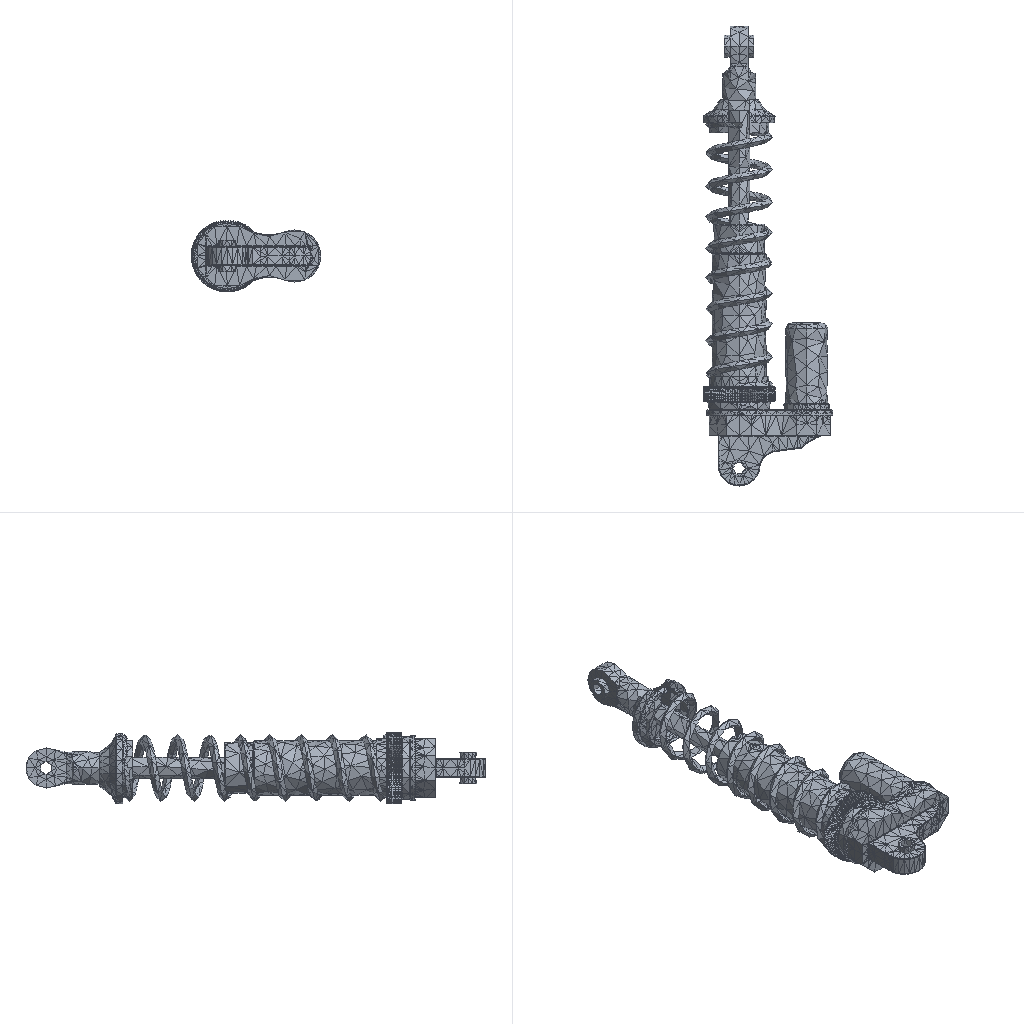Simulation study | ansys workbench
Set-up summary:
category,name,step,type,value,unit,region
solver,ansys_mapdl
solver,version,,,21.1
solver,version,,,21.1
solver,version,,,21.1
solver,version,,,21.1
solver,version,,,21.1
solver,version,,,21.1
solver,version,,,21.1
units,MPA,,stated
analysis,deck1,,transient,transient
load_step,requested,,,1
analysis,nlgeom,,,True
mesh,nodes,,,36272
mesh,elements,,,22272
element_type,ANSYS 187 (type 1),,solid,16919
element_type,ANSYS 187 (type 2),,solid,684
element_type,ANSYS 187 (type 3),,solid,554
element_type,ANSYS 187 (type 4),,solid,953
element_type,ANSYS 174 (type 5),,contact,35
element_type,ANSYS 170 (type 6),,target,35
element_type,ANSYS 174 (type 7),,contact,14
element_type,ANSYS 170 (type 8),,target,14
element_type,ANSYS 174 (type 9),,contact,1251
element_type,ANSYS 170 (type 10),,target,1251
element_type,ANSYS 174 (type 11),,contact,68
element_type,ANSYS 170 (type 12),,target,68
element_type,ANSYS 174 (type 13),,contact,148
element_type,ANSYS 170 (type 14),,target,148
element_type,ANSYS 154 (type 15),,surface,130
load,load commands in deck,,count,1
bc,support commands in deck,,count,1
named_set,_FIXEDSU,,component
analysis,deck2,,static,static
load_step,requested,,,1
analysis,nlgeom,,,False
mesh,nodes,,,36272
mesh,elements,,,22462
element_type,ANSYS 291 (type 1),,thermal_solid,16919
element_type,ANSYS 291 (type 2),,thermal_solid,684
element_type,ANSYS 291 (type 3),,thermal_solid,554
element_type,ANSYS 291 (type 4),,thermal_solid,953
element_type,ANSYS 174 (type 5),,contact,35
element_type,ANSYS 170 (type 6),,target,35
element_type,ANSYS 174 (type 7),,contact,14
element_type,ANSYS 170 (type 8),,target,14
element_type,ANSYS 174 (type 9),,contact,1251
element_type,ANSYS 170 (type 10),,target,1251
element_type,ANSYS 174 (type 11),,contact,68
element_type,ANSYS 170 (type 12),,target,68
element_type,ANSYS 174 (type 13),,contact,148
element_type,ANSYS 170 (type 14),,target,148
element_type,ANSYS 152 (type 15),,surface,320
load,load commands in deck,,count,4
bc,support commands in deck,,count,3
named_set,_CM86,,component
named_set,_CM95,,component
named_set,_ELMISC,,component
analysis,deck3,,modal,modal
load_step,requested,,,2
analysis,nlgeom,,,False
mesh,nodes,,,0
mesh,elements,,,0
load,load commands in deck,,count,0
bc,support commands in deck,,count,0
analysis,deck4,,modal,HARM; modal
load_step,requested,,,4
analysis,nlgeom,,,False
mesh,nodes,,,36272
mesh,elements,,,22272
element_type,ANSYS 187 (type 1),,solid,16919
element_type,ANSYS 187 (type 2),,solid,684
element_type,ANSYS 187 (type 3),,solid,554
element_type,ANSYS 187 (type 4),,solid,953
element_type,ANSYS 174 (type 5),,contact,35
element_type,ANSYS 170 (type 6),,target,35
element_type,ANSYS 174 (type 7),,contact,14
element_type,ANSYS 170 (type 8),,target,14
element_type,ANSYS 174 (type 9),,contact,1251
element_type,ANSYS 170 (type 10),,target,1251
element_type,ANSYS 174 (type 11),,contact,68
element_type,ANSYS 170 (type 12),,target,68
element_type,ANSYS 174 (type 13),,contact,148
element_type,ANSYS 170 (type 14),,target,148
element_type,ANSYS 154 (type 15),,surface,130
load,load commands in deck,,count,2
bc,support commands in deck,,count,0
analysis,deck5,,static,static
load_step,requested,,,1
analysis,nlgeom,,,False
mesh,nodes,,,36272
mesh,elements,,,22272
element_type,ANSYS 187 (type 1),,solid,16919
element_type,ANSYS 187 (type 2),,solid,684
element_type,ANSYS 187 (type 3),,solid,554
element_type,ANSYS 187 (type 4),,solid,953
element_type,ANSYS 174 (type 5),,contact,35
element_type,ANSYS 170 (type 6),,target,35
element_type,ANSYS 174 (type 7),,contact,14
element_type,ANSYS 170 (type 8),,target,14
element_type,ANSYS 174 (type 9),,contact,1251
element_type,ANSYS 170 (type 10),,target,1251
element_type,ANSYS 174 (type 11),,contact,68
element_type,ANSYS 170 (type 12),,target,68
element_type,ANSYS 174 (type 13),,contact,148
element_type,ANSYS 170 (type 14),,target,148
element_type,ANSYS 154 (type 15),,surface,130
load,load commands in deck,,count,1
bc,support commands in deck,,count,1
named_set,_CM53_FIXEDSU,,component
named_set,_FIXEDSU,,component
material,1,,in results
material,2,,in results
material,3,,in results
material,4,,in results
material,1,,in results
material,2,,in results
material,3,,in results
material,4,,in results
material,1,,in results
material,2,,in results
material,3,,in results
material,4,,in results
material,1,,in results
material,2,,in results
material,3,,in results
material,4,,in results
material,1,,in results
material,4,,in results
material,1,,in results
material,2,,in results
material,3,,in results
material,1,,in results
material,2,,in results
material,3,,in results
material,4,,in results
check,setup vs results,,match,130 surface effect element(s) are not in the reader's mesh and were not compared
check,setup vs results,,match,320 surface effect element(s) are not in the reader's mesh and were not compared
check,setup vs results,,match,130 surface effect element(s) are not in the reader's mesh and were not compared
check,setup vs results,,match,130 surface effect element(s) are not in the reader's mesh and were not compared
check,setup vs results,,match,130 surface effect element(s) are not in the reader's mesh and were not compared
Results summary:
result,analysis,,,static
result,last_loadstep,,,1
result,primary field,,,displacement
result,reaction total,1,FX,0.000822,N
result,reaction total,1,FY,81.914,N
result,reaction total,1,FZ,-11.71,N
result,mass,,,0.000104,"NMM: mm, ton, N, s, mV, mA, degC"
result,analysis,,,static
result,last_loadstep,,,1
result,primary field,,,temperature
result,mass,,,0.000104,"NMM: mm, ton, N, s, mV, mA, degC"
result,analysis,,,modal
result,last_loadstep,,,1
result,primary field,,,displacement
result,analysis,,,msup
result,last_loadstep,,,1
result,primary field,,,displacement
result,mass,,,0.000104,"NMM: mm, ton, N, s, mV, mA, degC"
result,analysis,,,static
result,last_loadstep,,,1
result,primary field,,,displacement
result,mass,,,5.5e-05,"NMM: mm, ton, N, s, mV, mA, degC"
result,analysis,,,static
result,last_loadstep,,,1
result,primary field,,,displacement
result,reaction total,1,FX,-9.1e-05,N
result,reaction total,1,FY,68.254,N
result,reaction total,1,FZ,-9.816,N
result,mass,,,4.9e-05,"NMM: mm, ton, N, s, mV, mA, degC"
result,analysis,,,static
result,last_loadstep,,,1
result,primary field,,,displacement
result,reaction total,1,FX,-9.1e-05,N
result,reaction total,1,FY,68.254,N
result,reaction total,1,FZ,-9.816,N
result,mass,,,0.000104,"NMM: mm, ton, N, s, mV, mA, degC"